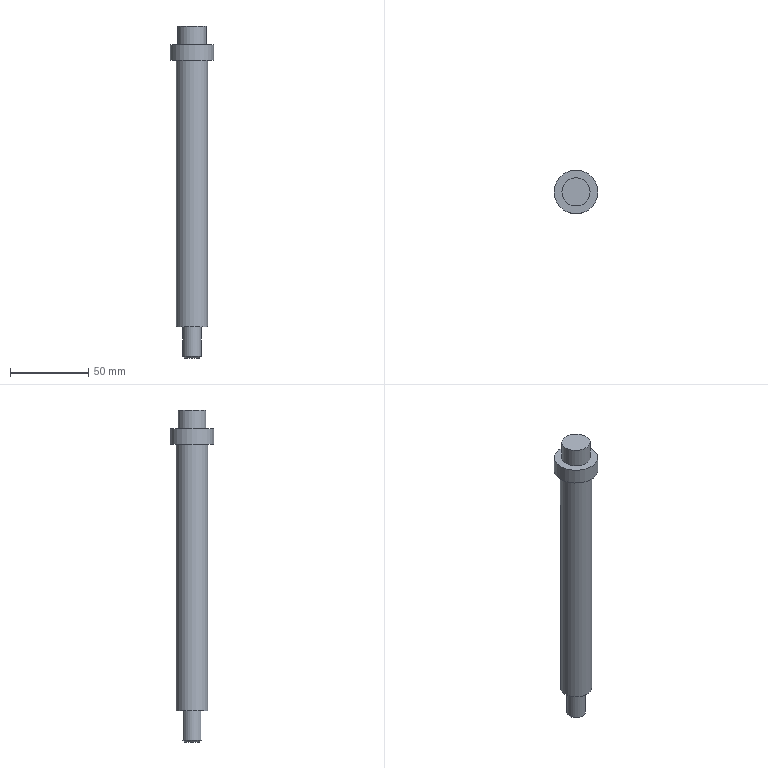Part | NX | features solid 2 | 1 solid | 10 faces | box 28 x 28 x 212 mm | volume 64862 mm3 | plane 5 | cylinder 4 | cone 1 | commonest cylinder face diameters 12 x1 18 x1 20 x1 28 x1
STEP:
#1=CARTESIAN_POINT('',(130.,-50.,45.));
#2=VERTEX_POINT('',#1);
#3=CARTESIAN_POINT('',(120.,-50.,45.));
#4=DIRECTION('',(0.,0.,1.));
#5=DIRECTION('',(1.,0.,0.));
#6=AXIS2_PLACEMENT_3D('',#3,#4,#5);
#7=CIRCLE('',#6,10.);
#8=EDGE_CURVE('',#2,#2,#7,.T.);
#9=ORIENTED_EDGE('',*,*,#8,.F.);
#10=EDGE_LOOP('',(#9));
#11=FACE_BOUND('',#10,.T.);
#12=CARTESIAN_POINT('',(114.,-50.,45.));
#13=VERTEX_POINT('',#12);
#14=CARTESIAN_POINT('',(120.,-50.,45.));
#15=DIRECTION('',(0.,0.,-1.));
#16=DIRECTION('',(-1.,0.,0.));
#17=AXIS2_PLACEMENT_3D('',#14,#15,#16);
#18=CIRCLE('',#17,6.);
#19=EDGE_CURVE('',#13,#13,#18,.T.);
#20=ORIENTED_EDGE('',*,*,#19,.F.);
#21=EDGE_LOOP('',(#20));
#22=FACE_BOUND('',#21,.T.);
#23=CARTESIAN_POINT('',(120.,-50.,45.));
#24=DIRECTION('',(0.,0.,-1.));
#25=DIRECTION('',(1.,0.,0.));
#26=AXIS2_PLACEMENT_3D('',#23,#24,#25);
#27=PLANE('',#26);
#28=ADVANCED_FACE('',(#11,#22),#27,.T.);
#29=CARTESIAN_POINT('',(134.,-50.,225.));
#30=VERTEX_POINT('',#29);
#31=CARTESIAN_POINT('',(120.,-50.,225.));
#32=DIRECTION('',(0.,0.,1.));
#33=DIRECTION('',(1.,0.,0.));
#34=AXIS2_PLACEMENT_3D('',#31,#32,#33);
#35=CIRCLE('',#34,14.);
#36=EDGE_CURVE('',#30,#30,#35,.T.);
#37=ORIENTED_EDGE('',*,*,#36,.T.);
#38=EDGE_LOOP('',(#37));
#39=FACE_BOUND('',#38,.T.);
#40=CARTESIAN_POINT('',(129.,-50.,225.));
#41=VERTEX_POINT('',#40);
#42=CARTESIAN_POINT('',(120.,-50.,225.));
#43=DIRECTION('',(0.,0.,1.));
#44=DIRECTION('',(1.,0.,0.));
#45=AXIS2_PLACEMENT_3D('',#42,#43,#44);
#46=CIRCLE('',#45,9.);
#47=EDGE_CURVE('',#41,#41,#46,.T.);
#48=ORIENTED_EDGE('',*,*,#47,.F.);
#49=EDGE_LOOP('',(#48));
#50=FACE_BOUND('',#49,.T.);
#51=CARTESIAN_POINT('',(120.,-50.,225.));
#52=DIRECTION('',(0.,0.,1.));
#53=DIRECTION('',(1.,0.,0.));
#54=AXIS2_PLACEMENT_3D('',#51,#52,#53);
#55=PLANE('',#54);
#56=ADVANCED_FACE('',(#39,#50),#55,.T.);
#57=CARTESIAN_POINT('',(130.,-50.,215.));
#58=VERTEX_POINT('',#57);
#59=CARTESIAN_POINT('',(120.,-50.,215.));
#60=DIRECTION('',(0.,0.,1.));
#61=DIRECTION('',(1.,0.,0.));
#62=AXIS2_PLACEMENT_3D('',#59,#60,#61);
#63=CIRCLE('',#62,10.);
#64=EDGE_CURVE('',#58,#58,#63,.T.);
#65=ORIENTED_EDGE('',*,*,#64,.F.);
#66=EDGE_LOOP('',(#65));
#67=FACE_BOUND('',#66,.T.);
#68=ORIENTED_EDGE('',*,*,#8,.T.);
#69=EDGE_LOOP('',(#68));
#70=FACE_BOUND('',#69,.T.);
#71=CARTESIAN_POINT('',(120.,-50.,185.));
#72=DIRECTION('',(0.,0.,-1.));
#73=DIRECTION('',(-1.,0.,0.));
#74=AXIS2_PLACEMENT_3D('',#71,#72,#73);
#75=CYLINDRICAL_SURFACE('',#74,10.);
#76=ADVANCED_FACE('',(#67,#70),#75,.T.);
#77=CARTESIAN_POINT('',(134.,-50.,215.));
#78=VERTEX_POINT('',#77);
#79=CARTESIAN_POINT('',(120.,-50.,215.));
#80=DIRECTION('',(0.,0.,1.));
#81=DIRECTION('',(1.,0.,0.));
#82=AXIS2_PLACEMENT_3D('',#79,#80,#81);
#83=CIRCLE('',#82,14.);
#84=EDGE_CURVE('',#78,#78,#83,.T.);
#85=ORIENTED_EDGE('',*,*,#84,.F.);
#86=EDGE_LOOP('',(#85));
#87=FACE_BOUND('',#86,.T.);
#88=ORIENTED_EDGE('',*,*,#64,.T.);
#89=EDGE_LOOP('',(#88));
#90=FACE_BOUND('',#89,.T.);
#91=CARTESIAN_POINT('',(120.,-50.,215.));
#92=DIRECTION('',(0.,0.,1.));
#93=DIRECTION('',(1.,0.,0.));
#94=AXIS2_PLACEMENT_3D('',#91,#92,#93);
#95=PLANE('',#94);
#96=ADVANCED_FACE('',(#87,#90),#95,.F.);
#97=ORIENTED_EDGE('',*,*,#84,.T.);
#98=EDGE_LOOP('',(#97));
#99=FACE_BOUND('',#98,.T.);
#100=ORIENTED_EDGE('',*,*,#36,.F.);
#101=EDGE_LOOP('',(#100));
#102=FACE_BOUND('',#101,.T.);
#103=CARTESIAN_POINT('',(120.,-50.,198.));
#104=DIRECTION('',(0.,0.,-1.));
#105=DIRECTION('',(-1.,0.,0.));
#106=AXIS2_PLACEMENT_3D('',#103,#104,#105);
#107=CYLINDRICAL_SURFACE('',#106,14.);
#108=ADVANCED_FACE('',(#99,#102),#107,.T.);
#109=CARTESIAN_POINT('',(129.,-50.,237.));
#110=VERTEX_POINT('',#109);
#111=CARTESIAN_POINT('',(120.,-50.,237.));
#112=DIRECTION('',(0.,0.,1.));
#113=DIRECTION('',(1.,0.,0.));
#114=AXIS2_PLACEMENT_3D('',#111,#112,#113);
#115=CIRCLE('',#114,9.);
#116=EDGE_CURVE('',#110,#110,#115,.T.);
#117=ORIENTED_EDGE('',*,*,#116,.F.);
#118=EDGE_LOOP('',(#117));
#119=FACE_BOUND('',#118,.T.);
#120=ORIENTED_EDGE('',*,*,#47,.T.);
#121=EDGE_LOOP('',(#120));
#122=FACE_BOUND('',#121,.T.);
#123=CARTESIAN_POINT('',(120.,-50.,222.));
#124=DIRECTION('',(0.,0.,-1.));
#125=DIRECTION('',(-1.,0.,0.));
#126=AXIS2_PLACEMENT_3D('',#123,#124,#125);
#127=CYLINDRICAL_SURFACE('',#126,9.);
#128=ADVANCED_FACE('',(#119,#122),#127,.T.);
#129=ORIENTED_EDGE('',*,*,#116,.T.);
#130=EDGE_LOOP('',(#129));
#131=FACE_BOUND('',#130,.T.);
#132=CARTESIAN_POINT('',(120.,-50.,237.));
#133=DIRECTION('',(0.,0.,1.));
#134=DIRECTION('',(1.,0.,0.));
#135=AXIS2_PLACEMENT_3D('',#132,#133,#134);
#136=PLANE('',#135);
#137=ADVANCED_FACE('',(#131),#136,.T.);
#138=CARTESIAN_POINT('',(126.,-50.,26.));
#139=VERTEX_POINT('',#138);
#140=CARTESIAN_POINT('',(120.,-50.,26.));
#141=DIRECTION('',(0.,0.,1.));
#142=DIRECTION('',(1.,0.,0.));
#143=AXIS2_PLACEMENT_3D('',#140,#141,#142);
#144=CIRCLE('',#143,6.);
#145=EDGE_CURVE('',#139,#139,#144,.T.);
#146=ORIENTED_EDGE('',*,*,#145,.T.);
#147=EDGE_LOOP('',(#146));
#148=FACE_BOUND('',#147,.T.);
#149=ORIENTED_EDGE('',*,*,#19,.T.);
#150=EDGE_LOOP('',(#149));
#151=FACE_BOUND('',#150,.T.);
#152=CARTESIAN_POINT('',(120.,-50.,45.));
#153=DIRECTION('',(0.,0.,-1.));
#154=DIRECTION('',(-1.,0.,0.));
#155=AXIS2_PLACEMENT_3D('',#152,#153,#154);
#156=CYLINDRICAL_SURFACE('',#155,6.);
#157=ADVANCED_FACE('',(#148,#151),#156,.T.);
#158=CARTESIAN_POINT('',(125.,-50.,25.));
#159=VERTEX_POINT('',#158);
#160=CARTESIAN_POINT('',(120.,-50.,25.));
#161=DIRECTION('',(0.,0.,1.));
#162=DIRECTION('',(1.,0.,0.));
#163=AXIS2_PLACEMENT_3D('',#160,#161,#162);
#164=CIRCLE('',#163,5.);
#165=EDGE_CURVE('',#159,#159,#164,.F.);
#166=ORIENTED_EDGE('',*,*,#165,.T.);
#167=EDGE_LOOP('',(#166));
#168=FACE_BOUND('',#167,.T.);
#169=CARTESIAN_POINT('',(120.,-50.,25.));
#170=DIRECTION('',(0.,0.,1.));
#171=DIRECTION('',(1.,0.,0.));
#172=AXIS2_PLACEMENT_3D('',#169,#170,#171);
#173=PLANE('',#172);
#174=ADVANCED_FACE('',(#168),#173,.F.);
#175=ORIENTED_EDGE('',*,*,#165,.F.);
#176=EDGE_LOOP('',(#175));
#177=FACE_BOUND('',#176,.T.);
#178=ORIENTED_EDGE('',*,*,#145,.F.);
#179=EDGE_LOOP('',(#178));
#180=FACE_BOUND('',#179,.T.);
#181=CARTESIAN_POINT('',(120.,-50.,26.));
#182=DIRECTION('',(0.,0.,1.));
#183=DIRECTION('',(1.,0.,0.));
#184=AXIS2_PLACEMENT_3D('',#181,#182,#183);
#185=CONICAL_SURFACE('',#184,6.,0.7854);
#186=ADVANCED_FACE('',(#177,#180),#185,.T.);
#187=CLOSED_SHELL('',(#28,#56,#76,#96,#108,#128,#137,#157,#174,#186));
#188=MANIFOLD_SOLID_BREP('',#187);
#189=(LENGTH_UNIT()NAMED_UNIT(*)SI_UNIT(.MILLI.,.METRE.));
#190=UNCERTAINTY_MEASURE_WITH_UNIT(LENGTH_MEASURE(0.00001),#189,'','');
#191=(NAMED_UNIT(*)PLANE_ANGLE_UNIT()SI_UNIT($,.RADIAN.));
#192=(NAMED_UNIT(*)SI_UNIT($,.STERADIAN.)SOLID_ANGLE_UNIT());
#193=(GEOMETRIC_REPRESENTATION_CONTEXT(3)GLOBAL_UNCERTAINTY_ASSIGNED_CONTEXT((#190))GLOBAL_UNIT_ASSIGNED_CONTEXT((#189,#191,#192))REPRESENTATION_CONTEXT('',''));
#194=ADVANCED_BREP_SHAPE_REPRESENTATION('',(#188),#193);